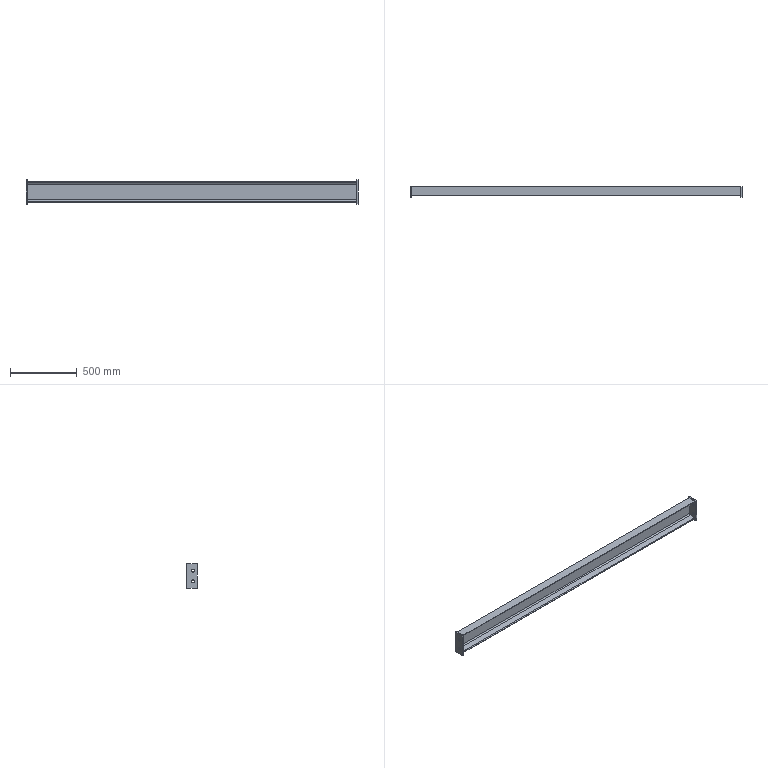Part | STEP file | Connecting beam 2_Default<As machined> | 3 solids | 34 faces | box 2484 x 75 x 180 mm | volume 5664884 mm3 | plane 22 | cylinder 12 | commonest cylinder face diameters 21 x8 10 x2 20 x2